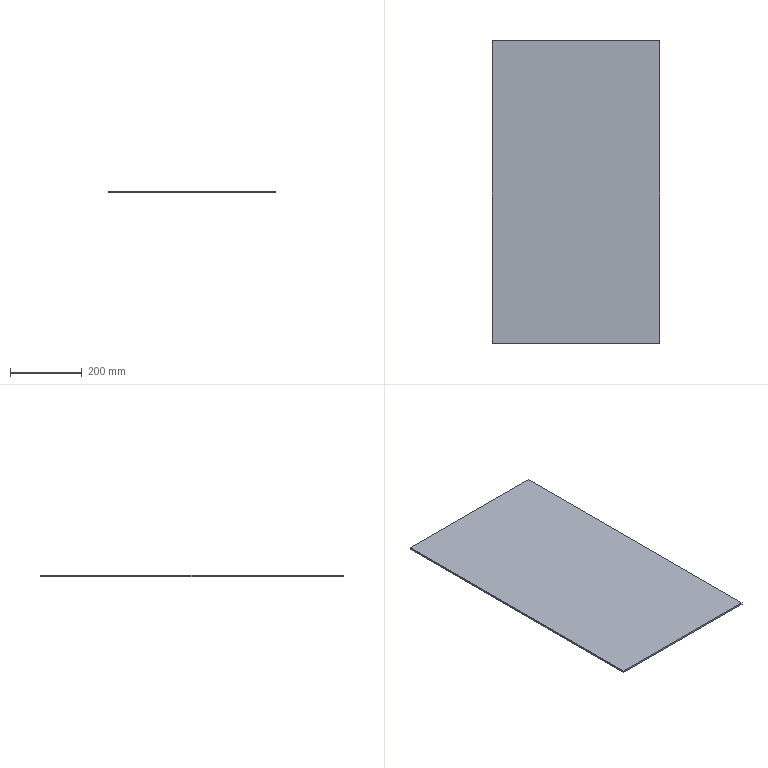Part | SolidWorks | features Extrusion 1, HoleWzd 1 | 1 solid | 6 faces | box 466 x 842 x 5 mm | volume 1961860 mm3 | plane 6
STEP:
#1=CARTESIAN_POINT('',(233.,-421.,0.));
#2=VERTEX_POINT('',#1);
#3=CARTESIAN_POINT('',(233.,421.,0.));
#4=VERTEX_POINT('',#3);
#5=CARTESIAN_POINT('',(233.,421.,0.));
#6=DIRECTION('',(0.,1.,0.));
#7=VECTOR('',#6,1000.);
#8=LINE('',#5,#7);
#9=EDGE_CURVE('',#2,#4,#8,.T.);
#10=ORIENTED_EDGE('',*,*,#9,.T.);
#11=CARTESIAN_POINT('',(233.,421.,5.));
#12=VERTEX_POINT('',#11);
#13=CARTESIAN_POINT('',(233.,421.,5.));
#14=DIRECTION('',(0.,0.,-1.));
#15=VECTOR('',#14,1000.);
#16=LINE('',#13,#15);
#17=EDGE_CURVE('',#12,#4,#16,.T.);
#18=ORIENTED_EDGE('',*,*,#17,.F.);
#19=CARTESIAN_POINT('',(233.,-421.,5.));
#20=VERTEX_POINT('',#19);
#21=CARTESIAN_POINT('',(233.,421.,5.));
#22=DIRECTION('',(0.,1.,0.));
#23=VECTOR('',#22,1000.);
#24=LINE('',#21,#23);
#25=EDGE_CURVE('',#20,#12,#24,.T.);
#26=ORIENTED_EDGE('',*,*,#25,.F.);
#27=CARTESIAN_POINT('',(233.,-421.,5.));
#28=DIRECTION('',(0.,0.,-1.));
#29=VECTOR('',#28,1000.);
#30=LINE('',#27,#29);
#31=EDGE_CURVE('',#20,#2,#30,.T.);
#32=ORIENTED_EDGE('',*,*,#31,.T.);
#33=EDGE_LOOP('',(#10,#18,#26,#32));
#34=FACE_OUTER_BOUND('',#33,.T.);
#35=CARTESIAN_POINT('',(233.,421.,5.));
#36=DIRECTION('',(-1.,0.,0.));
#37=DIRECTION('',(0.,-1.,0.));
#38=AXIS2_PLACEMENT_3D('',#35,#36,#37);
#39=PLANE('',#38);
#40=ADVANCED_FACE('',(#34),#39,.F.);
#41=CARTESIAN_POINT('',(-233.,421.,0.));
#42=VERTEX_POINT('',#41);
#43=CARTESIAN_POINT('',(-233.,421.,0.));
#44=DIRECTION('',(-1.,0.,0.));
#45=VECTOR('',#44,1000.);
#46=LINE('',#43,#45);
#47=EDGE_CURVE('',#4,#42,#46,.T.);
#48=ORIENTED_EDGE('',*,*,#47,.T.);
#49=CARTESIAN_POINT('',(-233.,421.,5.));
#50=VERTEX_POINT('',#49);
#51=CARTESIAN_POINT('',(-233.,421.,5.));
#52=DIRECTION('',(0.,0.,-1.));
#53=VECTOR('',#52,1000.);
#54=LINE('',#51,#53);
#55=EDGE_CURVE('',#50,#42,#54,.T.);
#56=ORIENTED_EDGE('',*,*,#55,.F.);
#57=CARTESIAN_POINT('',(-233.,421.,5.));
#58=DIRECTION('',(-1.,0.,0.));
#59=VECTOR('',#58,1000.);
#60=LINE('',#57,#59);
#61=EDGE_CURVE('',#12,#50,#60,.T.);
#62=ORIENTED_EDGE('',*,*,#61,.F.);
#63=ORIENTED_EDGE('',*,*,#17,.T.);
#64=EDGE_LOOP('',(#48,#56,#62,#63));
#65=FACE_OUTER_BOUND('',#64,.T.);
#66=CARTESIAN_POINT('',(-233.,421.,5.));
#67=DIRECTION('',(0.,-1.,0.));
#68=DIRECTION('',(0.,0.,-1.));
#69=AXIS2_PLACEMENT_3D('',#66,#67,#68);
#70=PLANE('',#69);
#71=ADVANCED_FACE('',(#65),#70,.F.);
#72=CARTESIAN_POINT('',(-233.,-421.,0.));
#73=VERTEX_POINT('',#72);
#74=CARTESIAN_POINT('',(-233.,421.,0.));
#75=DIRECTION('',(0.,-1.,0.));
#76=VECTOR('',#75,1000.);
#77=LINE('',#74,#76);
#78=EDGE_CURVE('',#42,#73,#77,.T.);
#79=ORIENTED_EDGE('',*,*,#78,.T.);
#80=CARTESIAN_POINT('',(-233.,-421.,5.));
#81=VERTEX_POINT('',#80);
#82=CARTESIAN_POINT('',(-233.,-421.,5.));
#83=DIRECTION('',(0.,0.,-1.));
#84=VECTOR('',#83,1000.);
#85=LINE('',#82,#84);
#86=EDGE_CURVE('',#81,#73,#85,.T.);
#87=ORIENTED_EDGE('',*,*,#86,.F.);
#88=CARTESIAN_POINT('',(-233.,421.,5.));
#89=DIRECTION('',(0.,-1.,0.));
#90=VECTOR('',#89,1000.);
#91=LINE('',#88,#90);
#92=EDGE_CURVE('',#50,#81,#91,.T.);
#93=ORIENTED_EDGE('',*,*,#92,.F.);
#94=ORIENTED_EDGE('',*,*,#55,.T.);
#95=EDGE_LOOP('',(#79,#87,#93,#94));
#96=FACE_OUTER_BOUND('',#95,.T.);
#97=CARTESIAN_POINT('',(-233.,421.,5.));
#98=DIRECTION('',(1.,0.,0.));
#99=DIRECTION('',(0.,1.,0.));
#100=AXIS2_PLACEMENT_3D('',#97,#98,#99);
#101=PLANE('',#100);
#102=ADVANCED_FACE('',(#96),#101,.F.);
#103=CARTESIAN_POINT('',(-233.,-421.,0.));
#104=DIRECTION('',(1.,0.,0.));
#105=VECTOR('',#104,1000.);
#106=LINE('',#103,#105);
#107=EDGE_CURVE('',#73,#2,#106,.T.);
#108=ORIENTED_EDGE('',*,*,#107,.T.);
#109=ORIENTED_EDGE('',*,*,#31,.F.);
#110=CARTESIAN_POINT('',(-233.,-421.,5.));
#111=DIRECTION('',(1.,0.,0.));
#112=VECTOR('',#111,1000.);
#113=LINE('',#110,#112);
#114=EDGE_CURVE('',#81,#20,#113,.T.);
#115=ORIENTED_EDGE('',*,*,#114,.F.);
#116=ORIENTED_EDGE('',*,*,#86,.T.);
#117=EDGE_LOOP('',(#108,#109,#115,#116));
#118=FACE_OUTER_BOUND('',#117,.T.);
#119=CARTESIAN_POINT('',(-233.,-421.,5.));
#120=DIRECTION('',(0.,1.,0.));
#121=DIRECTION('',(0.,0.,1.));
#122=AXIS2_PLACEMENT_3D('',#119,#120,#121);
#123=PLANE('',#122);
#124=ADVANCED_FACE('',(#118),#123,.F.);
#125=ORIENTED_EDGE('',*,*,#25,.T.);
#126=ORIENTED_EDGE('',*,*,#61,.T.);
#127=ORIENTED_EDGE('',*,*,#92,.T.);
#128=ORIENTED_EDGE('',*,*,#114,.T.);
#129=EDGE_LOOP('',(#125,#126,#127,#128));
#130=FACE_OUTER_BOUND('',#129,.T.);
#131=CARTESIAN_POINT('',(0.,0.,5.));
#132=DIRECTION('',(0.,0.,1.));
#133=DIRECTION('',(1.,0.,0.));
#134=AXIS2_PLACEMENT_3D('',#131,#132,#133);
#135=PLANE('',#134);
#136=ADVANCED_FACE('',(#130),#135,.T.);
#137=ORIENTED_EDGE('',*,*,#9,.F.);
#138=ORIENTED_EDGE('',*,*,#107,.F.);
#139=ORIENTED_EDGE('',*,*,#78,.F.);
#140=ORIENTED_EDGE('',*,*,#47,.F.);
#141=EDGE_LOOP('',(#137,#138,#139,#140));
#142=FACE_OUTER_BOUND('',#141,.T.);
#143=CARTESIAN_POINT('',(0.,0.,0.));
#144=DIRECTION('',(0.,0.,1.));
#145=DIRECTION('',(1.,0.,0.));
#146=AXIS2_PLACEMENT_3D('',#143,#144,#145);
#147=PLANE('',#146);
#148=ADVANCED_FACE('',(#142),#147,.F.);
#149=CLOSED_SHELL('',(#40,#71,#102,#124,#136,#148));
#150=MANIFOLD_SOLID_BREP('',#149);
#151=CARTESIAN_POINT('',(0.,0.,0.));
#152=DIRECTION('',(0.,0.,1.));
#153=DIRECTION('',(1.,0.,0.));
#154=AXIS2_PLACEMENT_3D('',#151,#152,#153);
#155=(LENGTH_UNIT()NAMED_UNIT(*)SI_UNIT(.MILLI.,.METRE.));
#156=UNCERTAINTY_MEASURE_WITH_UNIT(LENGTH_MEASURE(0.00001),#155,'','');
#157=(NAMED_UNIT(*)PLANE_ANGLE_UNIT()SI_UNIT($,.RADIAN.));
#158=(NAMED_UNIT(*)SI_UNIT($,.STERADIAN.)SOLID_ANGLE_UNIT());
#159=(GEOMETRIC_REPRESENTATION_CONTEXT(3)GLOBAL_UNCERTAINTY_ASSIGNED_CONTEXT((#156))GLOBAL_UNIT_ASSIGNED_CONTEXT((#155,#157,#158))REPRESENTATION_CONTEXT('',''));
#160=ADVANCED_BREP_SHAPE_REPRESENTATION('',(#150,#154),#159);